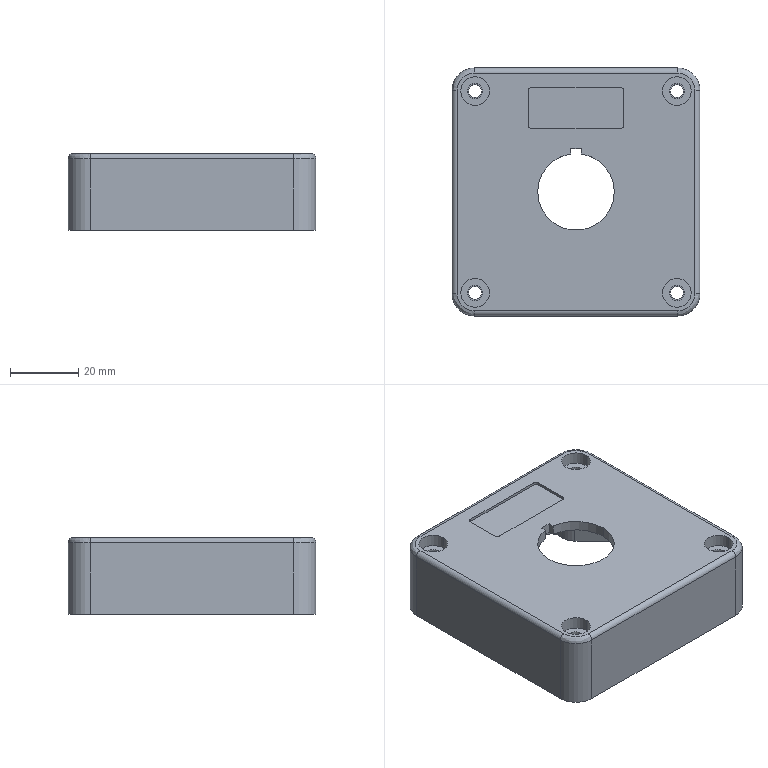Part | STEP file | APT8.315.0972 | 1 solid | 293 faces | box 72.5 x 72.5 x 22.5 mm | volume 32047 mm3 | plane 176 | cylinder 113 | spline 4 | commonest cylinder face diameters 3.8 x10 3 x8 4.5 x8 8.4 x8 11.6 x8 4.6 x6